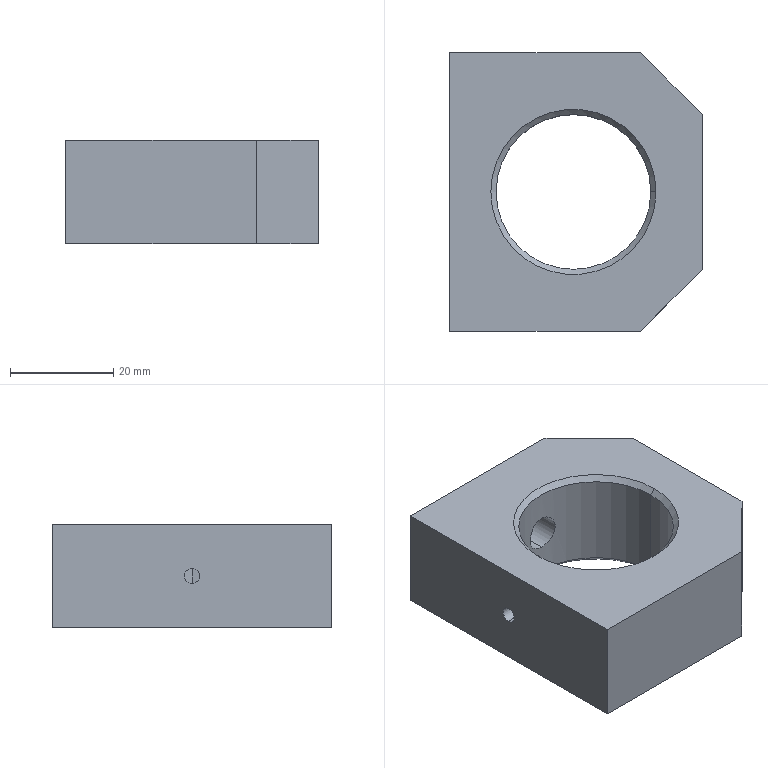Part | SolidWorks | features 3DProfileFeature 2, HoleWzd 2, Chamfer 1, Extrusion 1, ICE 1 | 1 solid | 18 faces | box 49 x 54 x 20 mm | volume 35303 mm3 | plane 8 | cylinder 6 | cone 4 | commonest cylinder face diameters 3 x2 6.8 x2 30 x2
STEP:
#1=CARTESIAN_POINT('',(-15.5,0.,8.5));
#2=VERTEX_POINT('',#1);
#3=CARTESIAN_POINT('',(-15.5,0.,11.5));
#4=VERTEX_POINT('',#3);
#5=CARTESIAN_POINT('',(-15.5,0.,8.5));
#6=CARTESIAN_POINT('',(-15.5,-0.1958,8.5));
#7=CARTESIAN_POINT('',(-15.496,-0.3932,8.539));
#8=CARTESIAN_POINT('',(-15.482,-0.7543,8.689));
#9=CARTESIAN_POINT('',(-15.472,-0.9216,8.8));
#10=CARTESIAN_POINT('',(-15.458,-1.129,9.008));
#11=CARTESIAN_POINT('',(-15.453,-1.192,9.085));
#12=CARTESIAN_POINT('',(-15.444,-1.301,9.248));
#13=CARTESIAN_POINT('',(-15.439,-1.348,9.334));
#14=CARTESIAN_POINT('',(-15.432,-1.423,9.515));
#15=CARTESIAN_POINT('',(-15.43,-1.452,9.611));
#16=CARTESIAN_POINT('',(-15.426,-1.49,9.802));
#17=CARTESIAN_POINT('',(-15.425,-1.5,9.9));
#18=CARTESIAN_POINT('',(-15.425,-1.5,10.197));
#19=CARTESIAN_POINT('',(-15.429,-1.461,10.392));
#20=CARTESIAN_POINT('',(-15.439,-1.348,10.664));
#21=CARTESIAN_POINT('',(-15.443,-1.302,10.751));
#22=CARTESIAN_POINT('',(-15.453,-1.194,10.914));
#23=CARTESIAN_POINT('',(-15.457,-1.13,10.991));
#24=CARTESIAN_POINT('',(-15.472,-0.9232,11.198));
#25=CARTESIAN_POINT('',(-15.482,-0.7561,11.31));
#26=CARTESIAN_POINT('',(-15.496,-0.3953,11.46));
#27=CARTESIAN_POINT('',(-15.5,-0.1983,11.5));
#28=CARTESIAN_POINT('',(-15.5,0.,11.5));
#29=B_SPLINE_CURVE_WITH_KNOTS('',3,(#5,#6,#7,#8,#9,#10,#11,#12,#13,#14,#15,#16,#17,#18,#19,#20,#21,#22,#23,#24,#25,#26,#27,#28),.UNSPECIFIED.,.F.,.F.,(4,2,2,2,2,2,2,2,2,2,2,4),(0.004693,0.005279,0.005865,0.006159,0.006452,0.006745,0.007038,0.007625,0.007918,0.008211,0.008798,0.009384),.UNSPECIFIED.);
#30=EDGE_CURVE('',#2,#4,#29,.T.);
#31=ORIENTED_EDGE('',*,*,#30,.F.);
#32=CARTESIAN_POINT('',(-24.5,0.,8.5));
#33=VERTEX_POINT('',#32);
#34=CARTESIAN_POINT('',(-24.5,0.,8.5));
#35=DIRECTION('',(-1.,0.,0.));
#36=VECTOR('',#35,1000.);
#37=LINE('',#34,#36);
#38=EDGE_CURVE('',#2,#33,#37,.T.);
#39=ORIENTED_EDGE('',*,*,#38,.T.);
#40=CARTESIAN_POINT('',(-24.5,0.,11.5));
#41=VERTEX_POINT('',#40);
#42=CARTESIAN_POINT('',(-24.5,0.,10.));
#43=DIRECTION('',(-1.,0.,0.));
#44=DIRECTION('',(0.,0.,1.));
#45=AXIS2_PLACEMENT_3D('',#42,#43,#44);
#46=CIRCLE('',#45,1.5);
#47=EDGE_CURVE('',#33,#41,#46,.T.);
#48=ORIENTED_EDGE('',*,*,#47,.T.);
#49=CARTESIAN_POINT('',(-24.5,0.,11.5));
#50=DIRECTION('',(-1.,0.,0.));
#51=VECTOR('',#50,1000.);
#52=LINE('',#49,#51);
#53=EDGE_CURVE('',#4,#41,#52,.T.);
#54=ORIENTED_EDGE('',*,*,#53,.F.);
#55=EDGE_LOOP('',(#31,#39,#48,#54));
#56=FACE_OUTER_BOUND('',#55,.T.);
#57=CARTESIAN_POINT('',(-24.5,0.,10.));
#58=DIRECTION('',(-1.,0.,0.));
#59=DIRECTION('',(0.,0.,1.));
#60=AXIS2_PLACEMENT_3D('',#57,#58,#59);
#61=CYLINDRICAL_SURFACE('',#60,1.5);
#62=ADVANCED_FACE('',(#56),#61,.F.);
#63=CARTESIAN_POINT('',(-15.5,0.,19.));
#64=VERTEX_POINT('',#63);
#65=CARTESIAN_POINT('',(14.5,0.,19.));
#66=VERTEX_POINT('',#65);
#67=CARTESIAN_POINT('',(-0.5,0.,19.));
#68=DIRECTION('',(0.,0.,1.));
#69=DIRECTION('',(1.,0.,0.));
#70=AXIS2_PLACEMENT_3D('',#67,#68,#69);
#71=CIRCLE('',#70,15.);
#72=EDGE_CURVE('',#64,#66,#71,.T.);
#73=ORIENTED_EDGE('',*,*,#72,.F.);
#74=CARTESIAN_POINT('',(-16.5,0.,20.));
#75=VERTEX_POINT('',#74);
#76=CARTESIAN_POINT('',(-15.5,0.,19.));
#77=DIRECTION('',(-0.7071,0.,0.7071));
#78=VECTOR('',#77,1000.);
#79=LINE('',#76,#78);
#80=EDGE_CURVE('',#64,#75,#79,.T.);
#81=ORIENTED_EDGE('',*,*,#80,.T.);
#82=CARTESIAN_POINT('',(15.5,0.,20.));
#83=VERTEX_POINT('',#82);
#84=CARTESIAN_POINT('',(-0.5,0.,20.));
#85=DIRECTION('',(0.,0.,-1.));
#86=DIRECTION('',(1.,0.,0.));
#87=AXIS2_PLACEMENT_3D('',#84,#85,#86);
#88=CIRCLE('',#87,16.);
#89=EDGE_CURVE('',#83,#75,#88,.T.);
#90=ORIENTED_EDGE('',*,*,#89,.F.);
#91=CARTESIAN_POINT('',(14.5,0.,19.));
#92=DIRECTION('',(0.7071,0.,0.7071));
#93=VECTOR('',#92,1000.);
#94=LINE('',#91,#93);
#95=EDGE_CURVE('',#66,#83,#94,.T.);
#96=ORIENTED_EDGE('',*,*,#95,.F.);
#97=EDGE_LOOP('',(#73,#81,#90,#96));
#98=FACE_OUTER_BOUND('',#97,.T.);
#99=CARTESIAN_POINT('',(-0.5,0.,19.));
#100=DIRECTION('',(0.,0.,1.));
#101=DIRECTION('',(1.,0.,0.));
#102=AXIS2_PLACEMENT_3D('',#99,#100,#101);
#103=CONICAL_SURFACE('',#102,15.,0.7854);
#104=ADVANCED_FACE('',(#98),#103,.F.);
#105=CARTESIAN_POINT('',(14.5,0.,1.));
#106=VERTEX_POINT('',#105);
#107=CARTESIAN_POINT('',(-15.5,0.,1.));
#108=VERTEX_POINT('',#107);
#109=CARTESIAN_POINT('',(-0.5,0.,1.));
#110=DIRECTION('',(0.,0.,-1.));
#111=DIRECTION('',(1.,0.,0.));
#112=AXIS2_PLACEMENT_3D('',#109,#110,#111);
#113=CIRCLE('',#112,15.);
#114=EDGE_CURVE('',#106,#108,#113,.T.);
#115=ORIENTED_EDGE('',*,*,#114,.F.);
#116=CARTESIAN_POINT('',(15.5,0.,0.));
#117=VERTEX_POINT('',#116);
#118=CARTESIAN_POINT('',(15.5,0.,0.));
#119=DIRECTION('',(0.7071,0.,-0.7071));
#120=VECTOR('',#119,1000.);
#121=LINE('',#118,#120);
#122=EDGE_CURVE('',#106,#117,#121,.T.);
#123=ORIENTED_EDGE('',*,*,#122,.T.);
#124=CARTESIAN_POINT('',(-16.5,0.,0.));
#125=VERTEX_POINT('',#124);
#126=CARTESIAN_POINT('',(-0.5,0.,0.));
#127=DIRECTION('',(0.,0.,1.));
#128=DIRECTION('',(1.,0.,0.));
#129=AXIS2_PLACEMENT_3D('',#126,#127,#128);
#130=CIRCLE('',#129,16.);
#131=EDGE_CURVE('',#125,#117,#130,.T.);
#132=ORIENTED_EDGE('',*,*,#131,.F.);
#133=CARTESIAN_POINT('',(-16.5,0.,0.));
#134=DIRECTION('',(-0.7071,0.,-0.7071));
#135=VECTOR('',#134,1000.);
#136=LINE('',#133,#135);
#137=EDGE_CURVE('',#108,#125,#136,.T.);
#138=ORIENTED_EDGE('',*,*,#137,.F.);
#139=EDGE_LOOP('',(#115,#123,#132,#138));
#140=FACE_OUTER_BOUND('',#139,.T.);
#141=CARTESIAN_POINT('',(-0.5,0.,0.));
#142=DIRECTION('',(0.,0.,-1.));
#143=DIRECTION('',(-1.,0.,0.));
#144=AXIS2_PLACEMENT_3D('',#141,#142,#143);
#145=CONICAL_SURFACE('',#144,16.,0.7854);
#146=ADVANCED_FACE('',(#140),#145,.F.);
#147=CARTESIAN_POINT('',(-0.5,15.,6.6));
#148=VERTEX_POINT('',#147);
#149=CARTESIAN_POINT('',(-0.5,15.,13.4));
#150=VERTEX_POINT('',#149);
#151=CARTESIAN_POINT('',(-0.5,15.,6.6));
#152=CARTESIAN_POINT('',(-0.7223,15.,6.6));
#153=CARTESIAN_POINT('',(-0.9437,14.995,6.622));
#154=CARTESIAN_POINT('',(-1.385,14.976,6.709));
#155=CARTESIAN_POINT('',(-1.598,14.961,6.775));
#156=CARTESIAN_POINT('',(-2.007,14.925,6.944));
#157=CARTESIAN_POINT('',(-2.206,14.904,7.051));
#158=CARTESIAN_POINT('',(-2.576,14.857,7.298));
#159=CARTESIAN_POINT('',(-2.746,14.832,7.438));
#160=CARTESIAN_POINT('',(-3.06,14.781,7.751));
#161=CARTESIAN_POINT('',(-3.203,14.755,7.926));
#162=CARTESIAN_POINT('',(-3.449,14.708,8.293));
#163=CARTESIAN_POINT('',(-3.554,14.686,8.488));
#164=CARTESIAN_POINT('',(-3.811,14.631,9.108));
#165=CARTESIAN_POINT('',(-3.9,14.61,9.55));
#166=CARTESIAN_POINT('',(-3.9,14.61,10.223));
#167=CARTESIAN_POINT('',(-3.878,14.615,10.444));
#168=CARTESIAN_POINT('',(-3.792,14.634,10.88));
#169=CARTESIAN_POINT('',(-3.726,14.649,11.097));
#170=CARTESIAN_POINT('',(-3.556,14.686,11.508));
#171=CARTESIAN_POINT('',(-3.451,14.707,11.703));
#172=CARTESIAN_POINT('',(-3.204,14.755,12.073));
#173=CARTESIAN_POINT('',(-3.062,14.78,12.246));
#174=CARTESIAN_POINT('',(-2.75,14.831,12.559));
#175=CARTESIAN_POINT('',(-2.578,14.857,12.7));
#176=CARTESIAN_POINT('',(-2.206,14.904,12.949));
#177=CARTESIAN_POINT('',(-2.011,14.925,13.054));
#178=CARTESIAN_POINT('',(-1.602,14.961,13.224));
#179=CARTESIAN_POINT('',(-1.386,14.975,13.29));
#180=CARTESIAN_POINT('',(-0.9477,14.995,13.378));
#181=CARTESIAN_POINT('',(-0.7254,15.,13.4));
#182=CARTESIAN_POINT('',(-0.5,15.,13.4));
#183=B_SPLINE_CURVE_WITH_KNOTS('',3,(#151,#152,#153,#154,#155,#156,#157,#158,#159,#160,#161,#162,#163,#164,#165,#166,#167,#168,#169,#170,#171,#172,#173,#174,#175,#176,#177,#178,#179,#180,#181,#182),.UNSPECIFIED.,.F.,.F.,(4,2,2,2,2,2,2,2,2,2,2,2,2,2,2,4),(0.01066,0.01133,0.012,0.01266,0.01333,0.014,0.01466,0.016,0.01666,0.01733,0.01799,0.01866,0.01933,0.01999,0.02066,0.02133),.UNSPECIFIED.);
#184=EDGE_CURVE('',#148,#150,#183,.T.);
#185=ORIENTED_EDGE('',*,*,#184,.F.);
#186=CARTESIAN_POINT('',(-0.5,27.,6.6));
#187=VERTEX_POINT('',#186);
#188=CARTESIAN_POINT('',(-0.5,27.,6.6));
#189=DIRECTION('',(0.,1.,0.));
#190=VECTOR('',#189,1000.);
#191=LINE('',#188,#190);
#192=EDGE_CURVE('',#148,#187,#191,.T.);
#193=ORIENTED_EDGE('',*,*,#192,.T.);
#194=CARTESIAN_POINT('',(-0.5,27.,13.4));
#195=VERTEX_POINT('',#194);
#196=CARTESIAN_POINT('',(-0.5,27.,10.));
#197=DIRECTION('',(0.,1.,0.));
#198=DIRECTION('',(0.,0.,1.));
#199=AXIS2_PLACEMENT_3D('',#196,#197,#198);
#200=CIRCLE('',#199,3.4);
#201=EDGE_CURVE('',#187,#195,#200,.T.);
#202=ORIENTED_EDGE('',*,*,#201,.T.);
#203=CARTESIAN_POINT('',(-0.5,27.,13.4));
#204=DIRECTION('',(0.,1.,0.));
#205=VECTOR('',#204,1000.);
#206=LINE('',#203,#205);
#207=EDGE_CURVE('',#150,#195,#206,.T.);
#208=ORIENTED_EDGE('',*,*,#207,.F.);
#209=EDGE_LOOP('',(#185,#193,#202,#208));
#210=FACE_OUTER_BOUND('',#209,.T.);
#211=CARTESIAN_POINT('',(-0.5,27.,10.));
#212=DIRECTION('',(0.,1.,0.));
#213=DIRECTION('',(0.,0.,1.));
#214=AXIS2_PLACEMENT_3D('',#211,#212,#213);
#215=CYLINDRICAL_SURFACE('',#214,3.4);
#216=ADVANCED_FACE('',(#210),#215,.F.);
#217=ORIENTED_EDGE('',*,*,#114,.T.);
#218=CARTESIAN_POINT('',(-15.5,0.,0.));
#219=DIRECTION('',(0.,0.,1.));
#220=VECTOR('',#219,1000.);
#221=LINE('',#218,#220);
#222=EDGE_CURVE('',#108,#2,#221,.T.);
#223=ORIENTED_EDGE('',*,*,#222,.T.);
#224=ORIENTED_EDGE('',*,*,#30,.T.);
#225=CARTESIAN_POINT('',(-15.5,0.,0.));
#226=DIRECTION('',(0.,0.,1.));
#227=VECTOR('',#226,1000.);
#228=LINE('',#225,#227);
#229=EDGE_CURVE('',#4,#64,#228,.T.);
#230=ORIENTED_EDGE('',*,*,#229,.T.);
#231=ORIENTED_EDGE('',*,*,#72,.T.);
#232=CARTESIAN_POINT('',(14.5,0.,0.));
#233=DIRECTION('',(0.,0.,1.));
#234=VECTOR('',#233,1000.);
#235=LINE('',#232,#234);
#236=EDGE_CURVE('',#106,#66,#235,.T.);
#237=ORIENTED_EDGE('',*,*,#236,.F.);
#238=EDGE_LOOP('',(#217,#223,#224,#230,#231,#237));
#239=FACE_OUTER_BOUND('',#238,.T.);
#240=CARTESIAN_POINT('',(-0.5,0.,0.));
#241=DIRECTION('',(0.,0.,1.));
#242=DIRECTION('',(1.,0.,0.));
#243=AXIS2_PLACEMENT_3D('',#240,#241,#242);
#244=CYLINDRICAL_SURFACE('',#243,15.);
#245=ADVANCED_FACE('',(#239),#244,.F.);
#246=CARTESIAN_POINT('',(-24.5,0.,10.));
#247=DIRECTION('',(-1.,0.,0.));
#248=DIRECTION('',(0.,0.,1.));
#249=AXIS2_PLACEMENT_3D('',#246,#247,#248);
#250=CIRCLE('',#249,1.5);
#251=EDGE_CURVE('',#41,#33,#250,.T.);
#252=ORIENTED_EDGE('',*,*,#251,.F.);
#253=ORIENTED_EDGE('',*,*,#47,.F.);
#254=EDGE_LOOP('',(#252,#253));
#255=FACE_BOUND('',#254,.T.);
#256=CARTESIAN_POINT('',(-24.5,27.,0.));
#257=VERTEX_POINT('',#256);
#258=CARTESIAN_POINT('',(-24.5,-27.,0.));
#259=VERTEX_POINT('',#258);
#260=CARTESIAN_POINT('',(-24.5,27.,0.));
#261=DIRECTION('',(0.,-1.,0.));
#262=VECTOR('',#261,1000.);
#263=LINE('',#260,#262);
#264=EDGE_CURVE('',#257,#259,#263,.T.);
#265=ORIENTED_EDGE('',*,*,#264,.T.);
#266=CARTESIAN_POINT('',(-24.5,-27.,20.));
#267=VERTEX_POINT('',#266);
#268=CARTESIAN_POINT('',(-24.5,-27.,20.));
#269=DIRECTION('',(0.,0.,-1.));
#270=VECTOR('',#269,1000.);
#271=LINE('',#268,#270);
#272=EDGE_CURVE('',#267,#259,#271,.T.);
#273=ORIENTED_EDGE('',*,*,#272,.F.);
#274=CARTESIAN_POINT('',(-24.5,27.,20.));
#275=VERTEX_POINT('',#274);
#276=CARTESIAN_POINT('',(-24.5,27.,20.));
#277=DIRECTION('',(0.,-1.,0.));
#278=VECTOR('',#277,1000.);
#279=LINE('',#276,#278);
#280=EDGE_CURVE('',#275,#267,#279,.T.);
#281=ORIENTED_EDGE('',*,*,#280,.F.);
#282=CARTESIAN_POINT('',(-24.5,27.,20.));
#283=DIRECTION('',(0.,0.,-1.));
#284=VECTOR('',#283,1000.);
#285=LINE('',#282,#284);
#286=EDGE_CURVE('',#275,#257,#285,.T.);
#287=ORIENTED_EDGE('',*,*,#286,.T.);
#288=EDGE_LOOP('',(#265,#273,#281,#287));
#289=FACE_OUTER_BOUND('',#288,.T.);
#290=CARTESIAN_POINT('',(-24.5,27.,20.));
#291=DIRECTION('',(1.,0.,0.));
#292=DIRECTION('',(0.,1.,0.));
#293=AXIS2_PLACEMENT_3D('',#290,#291,#292);
#294=PLANE('',#293);
#295=ADVANCED_FACE('',(#255,#289),#294,.F.);
#296=CARTESIAN_POINT('',(12.5,-27.,0.));
#297=VERTEX_POINT('',#296);
#298=CARTESIAN_POINT('',(-24.5,-27.,0.));
#299=DIRECTION('',(1.,0.,0.));
#300=VECTOR('',#299,1000.);
#301=LINE('',#298,#300);
#302=EDGE_CURVE('',#259,#297,#301,.T.);
#303=ORIENTED_EDGE('',*,*,#302,.T.);
#304=CARTESIAN_POINT('',(12.5,-27.,20.));
#305=VERTEX_POINT('',#304);
#306=CARTESIAN_POINT('',(12.5,-27.,20.));
#307=DIRECTION('',(0.,0.,-1.));
#308=VECTOR('',#307,1000.);
#309=LINE('',#306,#308);
#310=EDGE_CURVE('',#305,#297,#309,.T.);
#311=ORIENTED_EDGE('',*,*,#310,.F.);
#312=CARTESIAN_POINT('',(-24.5,-27.,20.));
#313=DIRECTION('',(1.,0.,0.));
#314=VECTOR('',#313,1000.);
#315=LINE('',#312,#314);
#316=EDGE_CURVE('',#267,#305,#315,.T.);
#317=ORIENTED_EDGE('',*,*,#316,.F.);
#318=ORIENTED_EDGE('',*,*,#272,.T.);
#319=EDGE_LOOP('',(#303,#311,#317,#318));
#320=FACE_OUTER_BOUND('',#319,.T.);
#321=CARTESIAN_POINT('',(-24.5,-27.,20.));
#322=DIRECTION('',(0.,1.,0.));
#323=DIRECTION('',(0.,0.,1.));
#324=AXIS2_PLACEMENT_3D('',#321,#322,#323);
#325=PLANE('',#324);
#326=ADVANCED_FACE('',(#320),#325,.F.);
#327=CARTESIAN_POINT('',(24.5,-15.,0.));
#328=VERTEX_POINT('',#327);
#329=CARTESIAN_POINT('',(12.5,-27.,0.));
#330=DIRECTION('',(0.7071,0.7071,0.));
#331=VECTOR('',#330,1000.);
#332=LINE('',#329,#331);
#333=EDGE_CURVE('',#297,#328,#332,.T.);
#334=ORIENTED_EDGE('',*,*,#333,.T.);
#335=CARTESIAN_POINT('',(24.5,-15.,20.));
#336=VERTEX_POINT('',#335);
#337=CARTESIAN_POINT('',(24.5,-15.,20.));
#338=DIRECTION('',(0.,0.,-1.));
#339=VECTOR('',#338,1000.);
#340=LINE('',#337,#339);
#341=EDGE_CURVE('',#336,#328,#340,.T.);
#342=ORIENTED_EDGE('',*,*,#341,.F.);
#343=CARTESIAN_POINT('',(12.5,-27.,20.));
#344=DIRECTION('',(0.7071,0.7071,0.));
#345=VECTOR('',#344,1000.);
#346=LINE('',#343,#345);
#347=EDGE_CURVE('',#305,#336,#346,.T.);
#348=ORIENTED_EDGE('',*,*,#347,.F.);
#349=ORIENTED_EDGE('',*,*,#310,.T.);
#350=EDGE_LOOP('',(#334,#342,#348,#349));
#351=FACE_OUTER_BOUND('',#350,.T.);
#352=CARTESIAN_POINT('',(12.5,-27.,20.));
#353=DIRECTION('',(-0.7071,0.7071,0.));
#354=DIRECTION('',(-0.7071,-0.7071,0.));
#355=AXIS2_PLACEMENT_3D('',#352,#353,#354);
#356=PLANE('',#355);
#357=ADVANCED_FACE('',(#351),#356,.F.);
#358=CARTESIAN_POINT('',(24.5,15.,0.));
#359=VERTEX_POINT('',#358);
#360=CARTESIAN_POINT('',(24.5,15.,0.));
#361=DIRECTION('',(0.,1.,0.));
#362=VECTOR('',#361,1000.);
#363=LINE('',#360,#362);
#364=EDGE_CURVE('',#328,#359,#363,.T.);
#365=ORIENTED_EDGE('',*,*,#364,.T.);
#366=CARTESIAN_POINT('',(24.5,15.,20.));
#367=VERTEX_POINT('',#366);
#368=CARTESIAN_POINT('',(24.5,15.,20.));
#369=DIRECTION('',(0.,0.,-1.));
#370=VECTOR('',#369,1000.);
#371=LINE('',#368,#370);
#372=EDGE_CURVE('',#367,#359,#371,.T.);
#373=ORIENTED_EDGE('',*,*,#372,.F.);
#374=CARTESIAN_POINT('',(24.5,15.,20.));
#375=DIRECTION('',(0.,1.,0.));
#376=VECTOR('',#375,1000.);
#377=LINE('',#374,#376);
#378=EDGE_CURVE('',#336,#367,#377,.T.);
#379=ORIENTED_EDGE('',*,*,#378,.F.);
#380=ORIENTED_EDGE('',*,*,#341,.T.);
#381=EDGE_LOOP('',(#365,#373,#379,#380));
#382=FACE_OUTER_BOUND('',#381,.T.);
#383=CARTESIAN_POINT('',(24.5,15.,20.));
#384=DIRECTION('',(-1.,0.,0.));
#385=DIRECTION('',(0.,-1.,0.));
#386=AXIS2_PLACEMENT_3D('',#383,#384,#385);
#387=PLANE('',#386);
#388=ADVANCED_FACE('',(#382),#387,.F.);
#389=CARTESIAN_POINT('',(12.5,27.,0.));
#390=VERTEX_POINT('',#389);
#391=CARTESIAN_POINT('',(12.5,27.,0.));
#392=DIRECTION('',(-0.7071,0.7071,0.));
#393=VECTOR('',#392,1000.);
#394=LINE('',#391,#393);
#395=EDGE_CURVE('',#359,#390,#394,.T.);
#396=ORIENTED_EDGE('',*,*,#395,.T.);
#397=CARTESIAN_POINT('',(12.5,27.,20.));
#398=VERTEX_POINT('',#397);
#399=CARTESIAN_POINT('',(12.5,27.,20.));
#400=DIRECTION('',(0.,0.,-1.));
#401=VECTOR('',#400,1000.);
#402=LINE('',#399,#401);
#403=EDGE_CURVE('',#398,#390,#402,.T.);
#404=ORIENTED_EDGE('',*,*,#403,.F.);
#405=CARTESIAN_POINT('',(12.5,27.,20.));
#406=DIRECTION('',(-0.7071,0.7071,0.));
#407=VECTOR('',#406,1000.);
#408=LINE('',#405,#407);
#409=EDGE_CURVE('',#367,#398,#408,.T.);
#410=ORIENTED_EDGE('',*,*,#409,.F.);
#411=ORIENTED_EDGE('',*,*,#372,.T.);
#412=EDGE_LOOP('',(#396,#404,#410,#411));
#413=FACE_OUTER_BOUND('',#412,.T.);
#414=CARTESIAN_POINT('',(12.5,27.,20.));
#415=DIRECTION('',(-0.7071,-0.7071,0.));
#416=DIRECTION('',(0.7071,-0.7071,0.));
#417=AXIS2_PLACEMENT_3D('',#414,#415,#416);
#418=PLANE('',#417);
#419=ADVANCED_FACE('',(#413),#418,.F.);
#420=CARTESIAN_POINT('',(-0.5,27.,10.));
#421=DIRECTION('',(0.,1.,0.));
#422=DIRECTION('',(0.,0.,1.));
#423=AXIS2_PLACEMENT_3D('',#420,#421,#422);
#424=CIRCLE('',#423,3.4);
#425=EDGE_CURVE('',#195,#187,#424,.T.);
#426=ORIENTED_EDGE('',*,*,#425,.F.);
#427=ORIENTED_EDGE('',*,*,#201,.F.);
#428=EDGE_LOOP('',(#426,#427));
#429=FACE_BOUND('',#428,.T.);
#430=CARTESIAN_POINT('',(-24.5,27.,0.));
#431=DIRECTION('',(-1.,0.,0.));
#432=VECTOR('',#431,1000.);
#433=LINE('',#430,#432);
#434=EDGE_CURVE('',#390,#257,#433,.T.);
#435=ORIENTED_EDGE('',*,*,#434,.T.);
#436=ORIENTED_EDGE('',*,*,#286,.F.);
#437=CARTESIAN_POINT('',(-24.5,27.,20.));
#438=DIRECTION('',(-1.,0.,0.));
#439=VECTOR('',#438,1000.);
#440=LINE('',#437,#439);
#441=EDGE_CURVE('',#398,#275,#440,.T.);
#442=ORIENTED_EDGE('',*,*,#441,.F.);
#443=ORIENTED_EDGE('',*,*,#403,.T.);
#444=EDGE_LOOP('',(#435,#436,#442,#443));
#445=FACE_OUTER_BOUND('',#444,.T.);
#446=CARTESIAN_POINT('',(-24.5,27.,20.));
#447=DIRECTION('',(0.,-1.,0.));
#448=DIRECTION('',(0.,0.,-1.));
#449=AXIS2_PLACEMENT_3D('',#446,#447,#448);
#450=PLANE('',#449);
#451=ADVANCED_FACE('',(#429,#445),#450,.F.);
#452=ORIENTED_EDGE('',*,*,#89,.T.);
#453=CARTESIAN_POINT('',(-0.5,0.,20.));
#454=DIRECTION('',(0.,0.,-1.));
#455=DIRECTION('',(1.,0.,0.));
#456=AXIS2_PLACEMENT_3D('',#453,#454,#455);
#457=CIRCLE('',#456,16.);
#458=EDGE_CURVE('',#75,#83,#457,.T.);
#459=ORIENTED_EDGE('',*,*,#458,.T.);
#460=EDGE_LOOP('',(#452,#459));
#461=FACE_BOUND('',#460,.T.);
#462=ORIENTED_EDGE('',*,*,#280,.T.);
#463=ORIENTED_EDGE('',*,*,#316,.T.);
#464=ORIENTED_EDGE('',*,*,#347,.T.);
#465=ORIENTED_EDGE('',*,*,#378,.T.);
#466=ORIENTED_EDGE('',*,*,#409,.T.);
#467=ORIENTED_EDGE('',*,*,#441,.T.);
#468=EDGE_LOOP('',(#462,#463,#464,#465,#466,#467));
#469=FACE_OUTER_BOUND('',#468,.T.);
#470=CARTESIAN_POINT('',(0.,0.,20.));
#471=DIRECTION('',(0.,0.,1.));
#472=DIRECTION('',(1.,0.,0.));
#473=AXIS2_PLACEMENT_3D('',#470,#471,#472);
#474=PLANE('',#473);
#475=ADVANCED_FACE('',(#461,#469),#474,.T.);
#476=ORIENTED_EDGE('',*,*,#131,.T.);
#477=CARTESIAN_POINT('',(-0.5,0.,0.));
#478=DIRECTION('',(0.,0.,1.));
#479=DIRECTION('',(1.,0.,0.));
#480=AXIS2_PLACEMENT_3D('',#477,#478,#479);
#481=CIRCLE('',#480,16.);
#482=EDGE_CURVE('',#117,#125,#481,.T.);
#483=ORIENTED_EDGE('',*,*,#482,.T.);
#484=EDGE_LOOP('',(#476,#483));
#485=FACE_BOUND('',#484,.T.);
#486=ORIENTED_EDGE('',*,*,#264,.F.);
#487=ORIENTED_EDGE('',*,*,#434,.F.);
#488=ORIENTED_EDGE('',*,*,#395,.F.);
#489=ORIENTED_EDGE('',*,*,#364,.F.);
#490=ORIENTED_EDGE('',*,*,#333,.F.);
#491=ORIENTED_EDGE('',*,*,#302,.F.);
#492=EDGE_LOOP('',(#486,#487,#488,#489,#490,#491));
#493=FACE_OUTER_BOUND('',#492,.T.);
#494=CARTESIAN_POINT('',(0.,0.,0.));
#495=DIRECTION('',(0.,0.,1.));
#496=DIRECTION('',(1.,0.,0.));
#497=AXIS2_PLACEMENT_3D('',#494,#495,#496);
#498=PLANE('',#497);
#499=ADVANCED_FACE('',(#485,#493),#498,.F.);
#500=ORIENTED_EDGE('',*,*,#222,.F.);
#501=CARTESIAN_POINT('',(-0.5,0.,1.));
#502=DIRECTION('',(0.,0.,-1.));
#503=DIRECTION('',(1.,0.,0.));
#504=AXIS2_PLACEMENT_3D('',#501,#502,#503);
#505=CIRCLE('',#504,15.);
#506=EDGE_CURVE('',#108,#106,#505,.T.);
#507=ORIENTED_EDGE('',*,*,#506,.T.);
#508=ORIENTED_EDGE('',*,*,#236,.T.);
#509=CARTESIAN_POINT('',(-0.5,0.,19.));
#510=DIRECTION('',(0.,0.,1.));
#511=DIRECTION('',(1.,0.,0.));
#512=AXIS2_PLACEMENT_3D('',#509,#510,#511);
#513=CIRCLE('',#512,15.);
#514=EDGE_CURVE('',#66,#64,#513,.T.);
#515=ORIENTED_EDGE('',*,*,#514,.T.);
#516=ORIENTED_EDGE('',*,*,#229,.F.);
#517=CARTESIAN_POINT('',(-15.5,0.,11.5));
#518=CARTESIAN_POINT('',(-15.5,0.09918,11.5));
#519=CARTESIAN_POINT('',(-15.499,0.1967,11.49));
#520=CARTESIAN_POINT('',(-15.495,0.3885,11.452));
#521=CARTESIAN_POINT('',(-15.492,0.4838,11.423));
#522=CARTESIAN_POINT('',(-15.486,0.6654,11.348));
#523=CARTESIAN_POINT('',(-15.481,0.7516,11.302));
#524=CARTESIAN_POINT('',(-15.472,0.9146,11.193));
#525=CARTESIAN_POINT('',(-15.467,0.9917,11.13));
#526=CARTESIAN_POINT('',(-15.453,1.199,10.922));
#527=CARTESIAN_POINT('',(-15.443,1.311,10.755));
#528=CARTESIAN_POINT('',(-15.429,1.46,10.394));
#529=CARTESIAN_POINT('',(-15.425,1.5,10.196));
#530=CARTESIAN_POINT('',(-15.425,1.5,9.903));
#531=CARTESIAN_POINT('',(-15.426,1.49,9.803));
#532=CARTESIAN_POINT('',(-15.43,1.452,9.611));
#533=CARTESIAN_POINT('',(-15.432,1.424,9.517));
#534=CARTESIAN_POINT('',(-15.439,1.348,9.336));
#535=CARTESIAN_POINT('',(-15.444,1.301,9.248));
#536=CARTESIAN_POINT('',(-15.453,1.193,9.085));
#537=CARTESIAN_POINT('',(-15.457,1.131,9.01));
#538=CARTESIAN_POINT('',(-15.467,0.9908,8.869));
#539=CARTESIAN_POINT('',(-15.472,0.9151,8.807));
#540=CARTESIAN_POINT('',(-15.481,0.7527,8.699));
#541=CARTESIAN_POINT('',(-15.486,0.6649,8.652));
#542=CARTESIAN_POINT('',(-15.492,0.4833,8.577));
#543=CARTESIAN_POINT('',(-15.495,0.3897,8.548));
#544=CARTESIAN_POINT('',(-15.499,0.1974,8.51));
#545=CARTESIAN_POINT('',(-15.5,0.09793,8.5));
#546=CARTESIAN_POINT('',(-15.5,0.,8.5));
#547=B_SPLINE_CURVE_WITH_KNOTS('',3,(#517,#518,#519,#520,#521,#522,#523,#524,#525,#526,#527,#528,#529,#530,#531,#532,#533,#534,#535,#536,#537,#538,#539,#540,#541,#542,#543,#544,#545,#546),.UNSPECIFIED.,.F.,.F.,(4,2,2,2,2,2,2,2,2,2,2,2,2,2,4),(0.,0.0002933,0.0005866,0.0008799,0.001173,0.00176,0.002346,0.00264,0.002933,0.003226,0.003519,0.003813,0.004106,0.004399,0.004693),.UNSPECIFIED.);
#548=EDGE_CURVE('',#4,#2,#547,.T.);
#549=ORIENTED_EDGE('',*,*,#548,.T.);
#550=EDGE_LOOP('',(#500,#507,#508,#515,#516,#549));
#551=FACE_OUTER_BOUND('',#550,.T.);
#552=CARTESIAN_POINT('',(-0.5,15.,13.4));
#553=CARTESIAN_POINT('',(-0.2746,15.,13.4));
#554=CARTESIAN_POINT('',(-0.05304,14.995,13.378));
#555=CARTESIAN_POINT('',(0.3825,14.976,13.291));
#556=CARTESIAN_POINT('',(0.5989,14.961,13.225));
#557=CARTESIAN_POINT('',(1.01,14.925,13.054));
#558=CARTESIAN_POINT('',(1.205,14.904,12.95));
#559=CARTESIAN_POINT('',(1.574,14.857,12.703));
#560=CARTESIAN_POINT('',(1.749,14.831,12.56));
#561=CARTESIAN_POINT('',(2.061,14.781,12.247));
#562=CARTESIAN_POINT('',(2.202,14.755,12.076));
#563=CARTESIAN_POINT('',(2.45,14.708,11.705));
#564=CARTESIAN_POINT('',(2.555,14.686,11.508));
#565=CARTESIAN_POINT('',(2.725,14.649,11.099));
#566=CARTESIAN_POINT('',(2.791,14.635,10.884));
#567=CARTESIAN_POINT('',(2.878,14.615,10.445));
#568=CARTESIAN_POINT('',(2.9,14.61,10.224));
#569=CARTESIAN_POINT('',(2.9,14.61,9.779));
#570=CARTESIAN_POINT('',(2.878,14.615,9.553));
#571=CARTESIAN_POINT('',(2.791,14.635,9.116));
#572=CARTESIAN_POINT('',(2.726,14.649,8.904));
#573=CARTESIAN_POINT('',(2.555,14.686,8.491));
#574=CARTESIAN_POINT('',(2.449,14.708,8.293));
#575=CARTESIAN_POINT('',(2.203,14.755,7.926));
#576=CARTESIAN_POINT('',(2.062,14.781,7.753));
#577=CARTESIAN_POINT('',(1.746,14.832,7.438));
#578=CARTESIAN_POINT('',(1.575,14.857,7.298));
#579=CARTESIAN_POINT('',(1.207,14.904,7.052));
#580=CARTESIAN_POINT('',(1.008,14.925,6.945));
#581=CARTESIAN_POINT('',(0.5975,14.961,6.774));
#582=CARTESIAN_POINT('',(0.3855,14.975,6.71));
#583=CARTESIAN_POINT('',(-0.05196,14.995,6.622));
#584=CARTESIAN_POINT('',(-0.2777,15.,6.6));
#585=CARTESIAN_POINT('',(-0.5,15.,6.6));
#586=B_SPLINE_CURVE_WITH_KNOTS('',3,(#552,#553,#554,#555,#556,#557,#558,#559,#560,#561,#562,#563,#564,#565,#566,#567,#568,#569,#570,#571,#572,#573,#574,#575,#576,#577,#578,#579,#580,#581,#582,#583,#584,#585),.UNSPECIFIED.,.F.,.F.,(4,2,2,2,2,2,2,2,2,2,2,2,2,2,2,2,4),(0.,0.0006665,0.001333,0.002,0.002666,0.003333,0.003999,0.004666,0.005332,0.005999,0.006665,0.007332,0.007999,0.008665,0.009332,0.009998,0.01066),.UNSPECIFIED.);
#587=EDGE_CURVE('',#150,#148,#586,.T.);
#588=ORIENTED_EDGE('',*,*,#587,.T.);
#589=ORIENTED_EDGE('',*,*,#184,.T.);
#590=EDGE_LOOP('',(#588,#589));
#591=FACE_BOUND('',#590,.T.);
#592=CARTESIAN_POINT('',(-0.5,0.,0.));
#593=DIRECTION('',(0.,0.,1.));
#594=DIRECTION('',(1.,0.,0.));
#595=AXIS2_PLACEMENT_3D('',#592,#593,#594);
#596=CYLINDRICAL_SURFACE('',#595,15.);
#597=ADVANCED_FACE('',(#551,#591),#596,.F.);
#598=ORIENTED_EDGE('',*,*,#192,.F.);
#599=ORIENTED_EDGE('',*,*,#587,.F.);
#600=ORIENTED_EDGE('',*,*,#207,.T.);
#601=ORIENTED_EDGE('',*,*,#425,.T.);
#602=EDGE_LOOP('',(#598,#599,#600,#601));
#603=FACE_OUTER_BOUND('',#602,.T.);
#604=CARTESIAN_POINT('',(-0.5,27.,10.));
#605=DIRECTION('',(0.,1.,0.));
#606=DIRECTION('',(0.,0.,1.));
#607=AXIS2_PLACEMENT_3D('',#604,#605,#606);
#608=CYLINDRICAL_SURFACE('',#607,3.4);
#609=ADVANCED_FACE('',(#603),#608,.F.);
#610=ORIENTED_EDGE('',*,*,#122,.F.);
#611=ORIENTED_EDGE('',*,*,#506,.F.);
#612=ORIENTED_EDGE('',*,*,#137,.T.);
#613=ORIENTED_EDGE('',*,*,#482,.F.);
#614=EDGE_LOOP('',(#610,#611,#612,#613));
#615=FACE_OUTER_BOUND('',#614,.T.);
#616=CARTESIAN_POINT('',(-0.5,0.,0.));
#617=DIRECTION('',(0.,0.,-1.));
#618=DIRECTION('',(-1.,0.,0.));
#619=AXIS2_PLACEMENT_3D('',#616,#617,#618);
#620=CONICAL_SURFACE('',#619,16.,0.7854);
#621=ADVANCED_FACE('',(#615),#620,.F.);
#622=ORIENTED_EDGE('',*,*,#80,.F.);
#623=ORIENTED_EDGE('',*,*,#514,.F.);
#624=ORIENTED_EDGE('',*,*,#95,.T.);
#625=ORIENTED_EDGE('',*,*,#458,.F.);
#626=EDGE_LOOP('',(#622,#623,#624,#625));
#627=FACE_OUTER_BOUND('',#626,.T.);
#628=CARTESIAN_POINT('',(-0.5,0.,19.));
#629=DIRECTION('',(0.,0.,1.));
#630=DIRECTION('',(1.,0.,0.));
#631=AXIS2_PLACEMENT_3D('',#628,#629,#630);
#632=CONICAL_SURFACE('',#631,15.,0.7854);
#633=ADVANCED_FACE('',(#627),#632,.F.);
#634=ORIENTED_EDGE('',*,*,#38,.F.);
#635=ORIENTED_EDGE('',*,*,#548,.F.);
#636=ORIENTED_EDGE('',*,*,#53,.T.);
#637=ORIENTED_EDGE('',*,*,#251,.T.);
#638=EDGE_LOOP('',(#634,#635,#636,#637));
#639=FACE_OUTER_BOUND('',#638,.T.);
#640=CARTESIAN_POINT('',(-24.5,0.,10.));
#641=DIRECTION('',(-1.,0.,0.));
#642=DIRECTION('',(0.,0.,1.));
#643=AXIS2_PLACEMENT_3D('',#640,#641,#642);
#644=CYLINDRICAL_SURFACE('',#643,1.5);
#645=ADVANCED_FACE('',(#639),#644,.F.);
#646=CLOSED_SHELL('',(#62,#104,#146,#216,#245,#295,#326,#357,#388,#419,#451,#475,#499,#597,#609,#621,#633,#645));
#647=MANIFOLD_SOLID_BREP('',#646);
#648=CARTESIAN_POINT('',(0.,0.,0.));
#649=DIRECTION('',(0.,0.,1.));
#650=DIRECTION('',(1.,0.,0.));
#651=AXIS2_PLACEMENT_3D('',#648,#649,#650);
#652=(LENGTH_UNIT()NAMED_UNIT(*)SI_UNIT(.MILLI.,.METRE.));
#653=UNCERTAINTY_MEASURE_WITH_UNIT(LENGTH_MEASURE(0.00001),#652,'','');
#654=(NAMED_UNIT(*)PLANE_ANGLE_UNIT()SI_UNIT($,.RADIAN.));
#655=(NAMED_UNIT(*)SI_UNIT($,.STERADIAN.)SOLID_ANGLE_UNIT());
#656=(GEOMETRIC_REPRESENTATION_CONTEXT(3)GLOBAL_UNCERTAINTY_ASSIGNED_CONTEXT((#653))GLOBAL_UNIT_ASSIGNED_CONTEXT((#652,#654,#655))REPRESENTATION_CONTEXT('',''));
#657=ADVANCED_BREP_SHAPE_REPRESENTATION('',(#647,#651),#656);